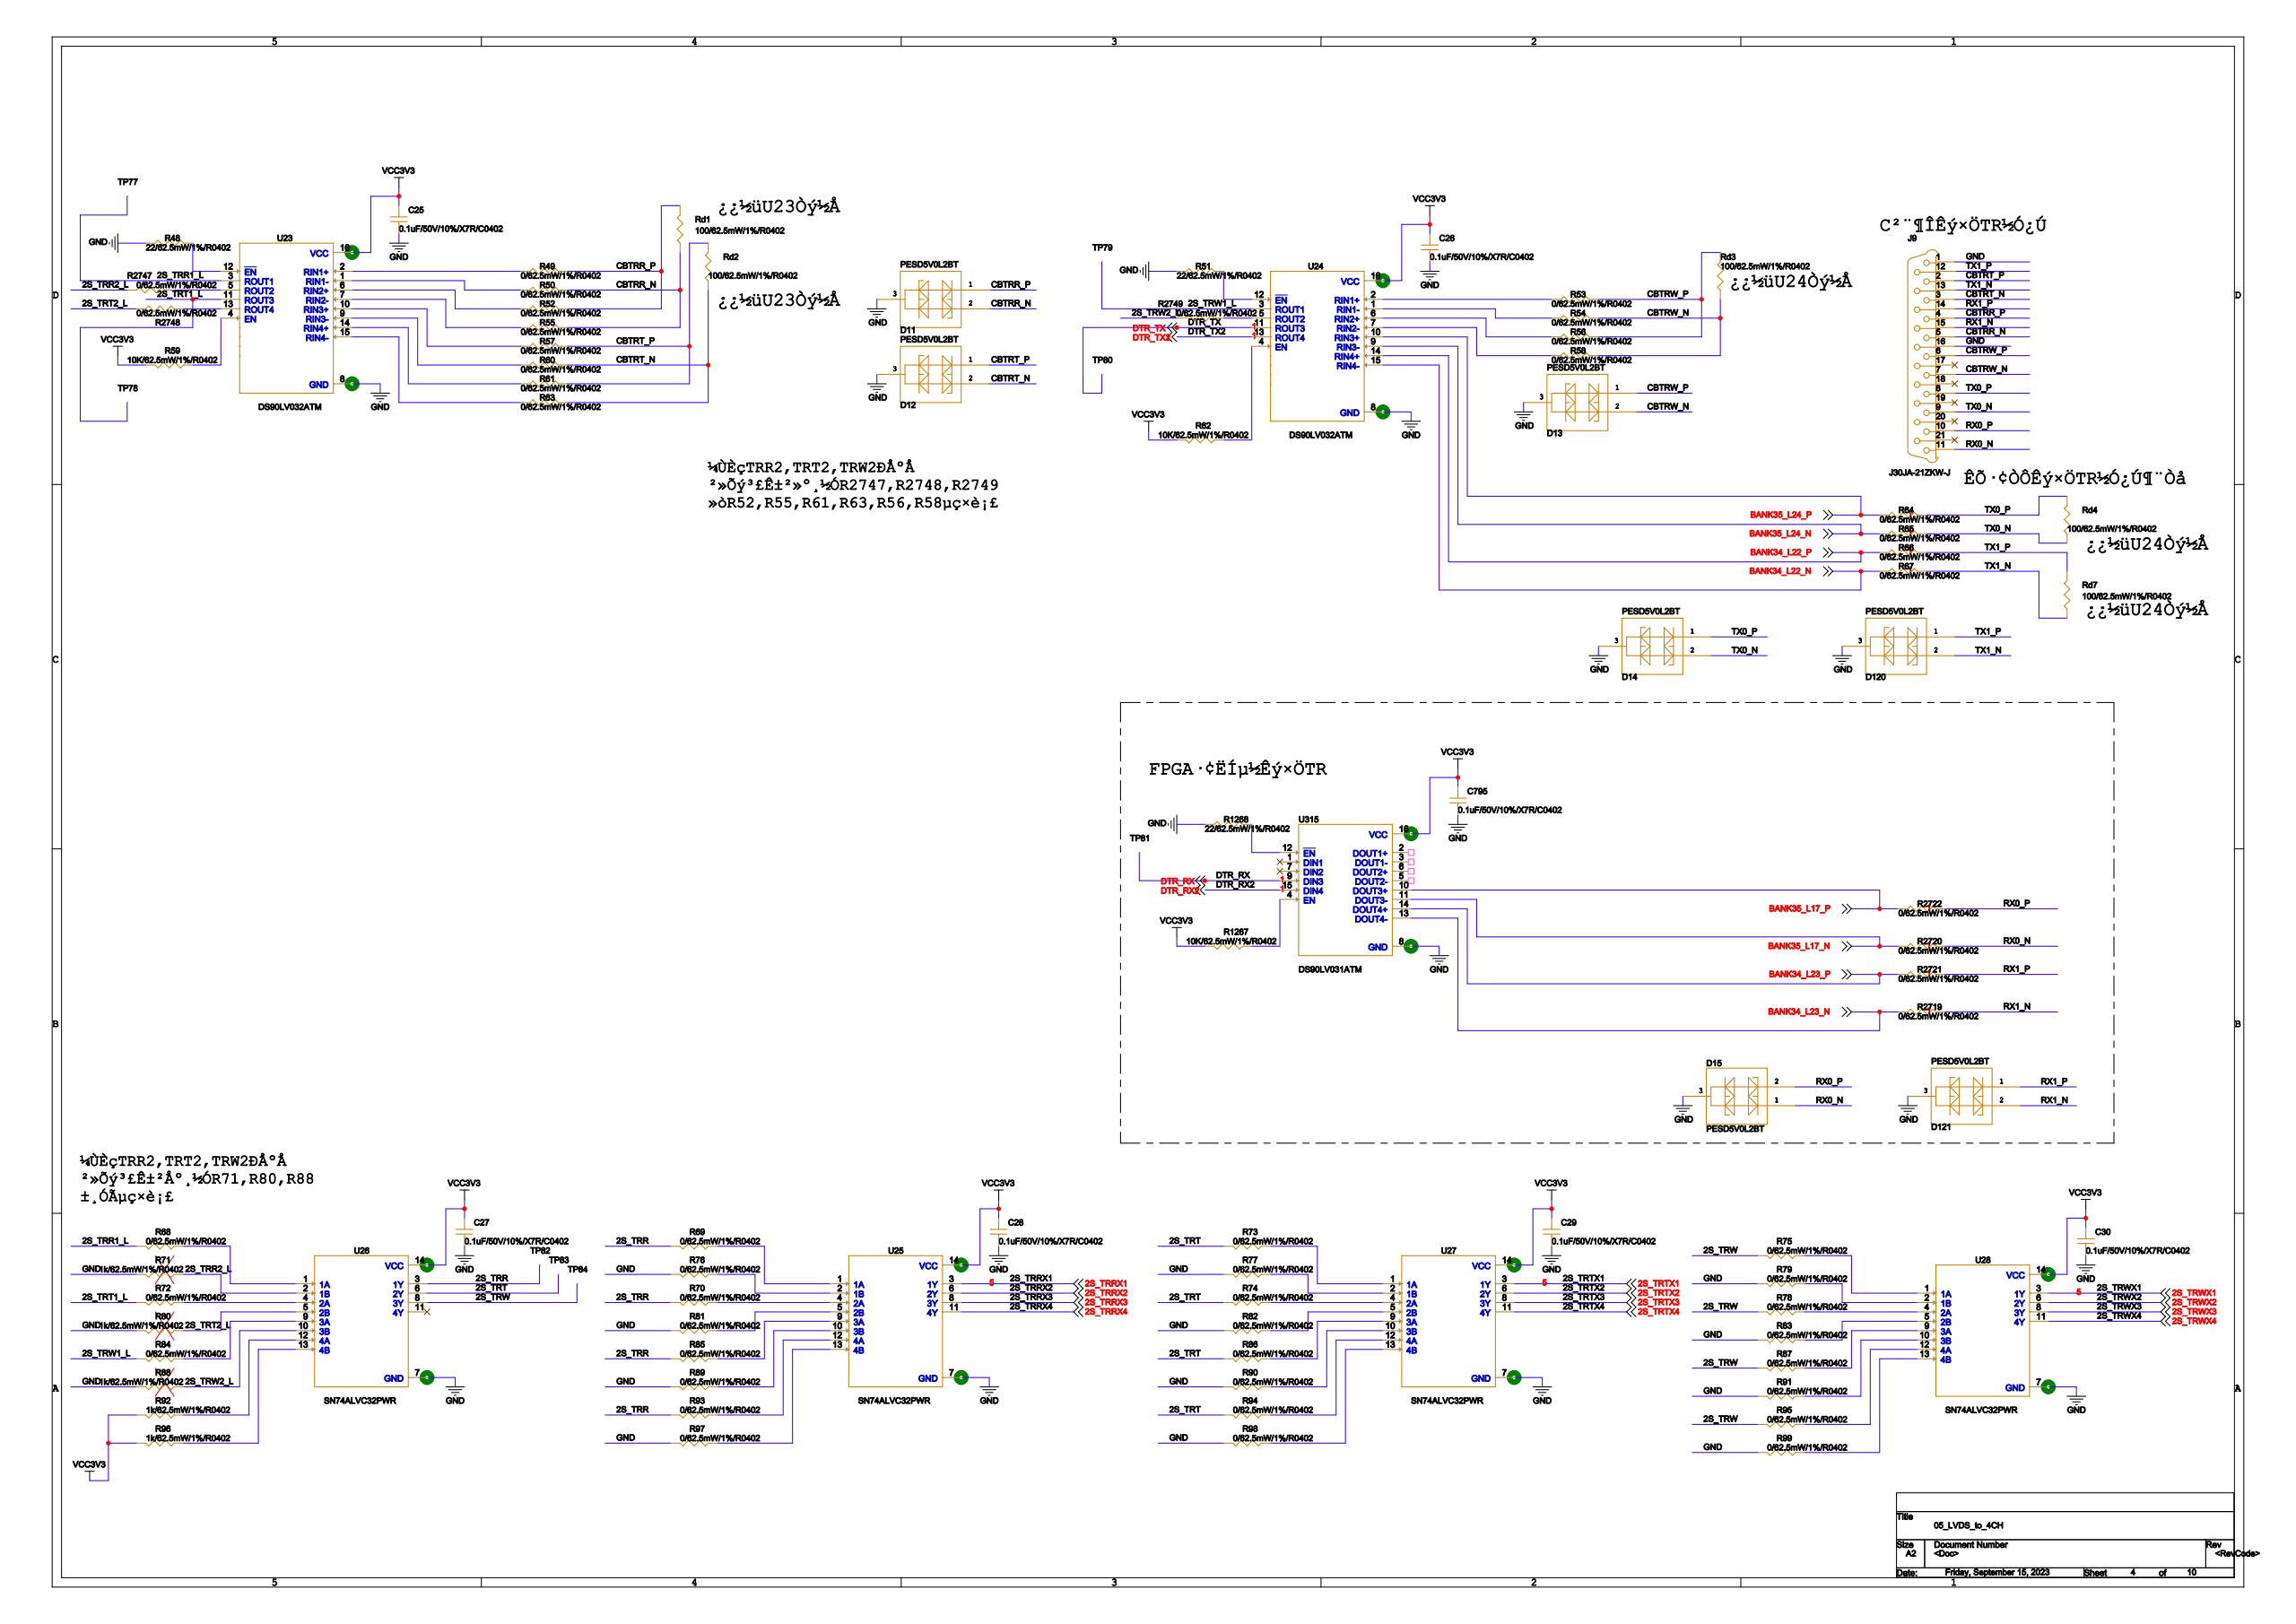Circuit board | Cadence Allegro | 634 parts | 645 nets | one sheet of the schematic
Parts on this sheet (reference | value | footprint):
C25 | 0.1uF/50V/10%/X7R/C0402 | 0402
C26 | 0.1uF/50V/10%/X7R/C0402 | 0402
C27 | 0.1uF/50V/10%/X7R/C0402 | 0402
C28 | 0.1uF/50V/10%/X7R/C0402 | 0402
C29 | 0.1uF/50V/10%/X7R/C0402 | 0402
C30 | 0.1uF/50V/10%/X7R/C0402 | 0402
C795 | 0.1uF/50V/10%/X7R/C0402 | 0402
D11 | PESD5V0L2BT | SOT23
D12 | PESD5V0L2BT | SOT23
D13 | PESD5V0L2BT | SOT23
D14 | PESD5V0L2BT | SOT23
D15 | PESD5V0L2BT | SOT23
D120 | PESD5V0L2BT | SOT23
D121 | PESD5V0L2BT | SOT23
J9 | J30JA-21ZKW-J | J30JA-21ZKW-J
R48 | 22/62.5mW/1%/R0402 | 0402
R49 | 0/62.5mW/1%/R0402 | 0402
R50 | 0/62.5mW/1%/R0402 | 0402
R51 | 22/62.5mW/1%/R0402 | 0402
R52 | 0/62.5mW/1%/R0402 | 0402
R53 | 0/62.5mW/1%/R0402 | 0402
R54 | 0/62.5mW/1%/R0402 | 0402
R55 | 0/62.5mW/1%/R0402 | 0402
R56 | 0/62.5mW/1%/R0402 | 0402
R57 | 0/62.5mW/1%/R0402 | 0402
R58 | 0/62.5mW/1%/R0402 | 0402
R59 | 10K/62.5mW/1%/R0402 | 0402
R60 | 0/62.5mW/1%/R0402 | 0402
R61 | 0/62.5mW/1%/R0402 | 0402
R62 | 10K/62.5mW/1%/R0402 | 0402
R63 | 0/62.5mW/1%/R0402 | 0402
R64 | 0/62.5mW/1%/R0402 | 0402
R65 | 0/62.5mW/1%/R0402 | 0402
R66 | 0/62.5mW/1%/R0402 | 0402
R67 | 0/62.5mW/1%/R0402 | 0402
R68 | 0/62.5mW/1%/R0402 | 0402
R69 | 0/62.5mW/1%/R0402 | 0402
R70 | 0/62.5mW/1%/R0402 | 0402
R71 | 1k/62.5mW/1%/R0402 | 0402
R72 | 0/62.5mW/1%/R0402 | 0402
R73 | 0/62.5mW/1%/R0402 | 0402
R74 | 0/62.5mW/1%/R0402 | 0402
R75 | 0/62.5mW/1%/R0402 | 0402
R76 | 0/62.5mW/1%/R0402 | 0402
R77 | 0/62.5mW/1%/R0402 | 0402
R78 | 0/62.5mW/1%/R0402 | 0402
R79 | 0/62.5mW/1%/R0402 | 0402
R80 | 1k/62.5mW/1%/R0402 | 0402
R81 | 0/62.5mW/1%/R0402 | 0402
R82 | 0/62.5mW/1%/R0402 | 0402
R83 | 0/62.5mW/1%/R0402 | 0402
R84 | 0/62.5mW/1%/R0402 | 0402
R85 | 0/62.5mW/1%/R0402 | 0402
R86 | 0/62.5mW/1%/R0402 | 0402
R87 | 0/62.5mW/1%/R0402 | 0402
R88 | 1k/62.5mW/1%/R0402 | 0402
R89 | 0/62.5mW/1%/R0402 | 0402
R90 | 0/62.5mW/1%/R0402 | 0402
R91 | 0/62.5mW/1%/R0402 | 0402
R92 | 1k/62.5mW/1%/R0402 | 0402
R93 | 0/62.5mW/1%/R0402 | 0402
R94 | 0/62.5mW/1%/R0402 | 0402
R95 | 0/62.5mW/1%/R0402 | 0402
R96 | 1k/62.5mW/1%/R0402 | 0402
R97 | 0/62.5mW/1%/R0402 | 0402
R98 | 0/62.5mW/1%/R0402 | 0402
R99 | 0/62.5mW/1%/R0402 | 0402
R1267 | 10K/62.5mW/1%/R0402 | 0402
R1268 | 22/62.5mW/1%/R0402 | 0402
R2719 | 0/62.5mW/1%/R0402 | 0402
R2720 | 0/62.5mW/1%/R0402 | 0402
R2721 | 0/62.5mW/1%/R0402 | 0402
R2722 | 0/62.5mW/1%/R0402 | 0402
R2747 | 0/62.5mW/1%/R0402 | 0402
R2748 | 0/62.5mW/1%/R0402 | 0402
R2749 | 0/62.5mW/1%/R0402 | 0402
TP77 | TEST POINT A | TEST_12MM
TP78 | TEST POINT A | TEST_12MM
TP79 | TEST POINT A | TEST_12MM
TP80 | TEST POINT A | TEST_12MM
TP81 | TEST POINT A | TEST_12MM
TP82 | TEST POINT A | TEST_12MM
TP83 | TEST POINT A | TEST_12MM
TP84 | TEST POINT A | TEST_12MM
U23 | DS90LV032ATM | SOIC127P600X175-16N
U24 | DS90LV032ATM | SOIC127P600X175-16N
U25 | SN74ALVC32PWR | SOP65P640X120-14N
U26 | SN74ALVC32PWR | SOP65P640X120-14N
U27 | SN74ALVC32PWR | SOP65P640X120-14N
U28 | SN74ALVC32PWR | SOP65P640X120-14N
U315 | DS90LV031ATM | SOIC127P600X175-16N
Nets of these parts (net: part-pin ...):
AGND: C25-2 C26-2 C27-2 C28-2 C29-2 C30-2 C795-2 D11-3 D12-3 D13-3 D14-3 D15-3 D120-3 D121-3 J9-1 J9-16 R48-2 R51-2 R71-1 R76-1 R77-1 R79-1 R80-1 R81-1 R82-1 R83-1 R88-1 R89-1 R90-1 R91-1 R97-1 R98-1 R99-1 R1268-2 U23-8 U24-8 U25-7 U26-7 U27-7 U28-7 U315-8
DTR_TX: TP80-1 U24-11
3.3V: C25-1 C26-1 C27-1 C28-1 C29-1 C30-1 C795-1 R59-1 R62-1 R92-1 R96-1 R1267-1 U23-16 U24-16 U25-14 U26-14 U27-14 U28-14 U315-16
DTR_TX2: U24-13
DTR_RX: TP81-1 U315-9
DTR_RX2: U315-15
BANK34_L23_P: R2721-2 U315-14
BANK34_L23_N: R2719-2 U315-13
BANK35_L17_P: R2722-2 U315-10
BANK35_L17_N: R2720-2 U315-11
BANK35_L24_P: R64-2 U24-10
BANK35_L24_N: R65-2 U24-9
BANK34_L22_P: R66-2 U24-14
BANK34_L22_N: R67-2 U24-15
2S_TRR2_L: R71-2 R2747-2 U26-2
2S_TRT2_L: R80-2 R2748-2 U26-5
2S_TRW2_L: R88-2 R2749-2 U26-10
N23948082: R92-2 U26-12
N23948113: R96-2 U26-13
N24593317: R1267-2 U315-4
N24593321: R1268-1 U315-12
TX1_P: D120-1 J9-12 R66-1
TX1_N: D120-2 J9-13 R67-1
CBTRR_P: D11-1 J9-4 R49-1 R52-1
CBTRR_N: D11-2 J9-5 R50-1 R55-1
CBTRT_P: D12-1 J9-2 R57-1 R61-1
CBTRT_N: D12-2 J9-3 R60-1 R63-1
CBTRW_P: D13-1 J9-6 R53-1 R56-1
CBTRW_N: D13-2 J9-7 R54-1 R58-1
TX0_P: D14-1 J9-8 R64-1
TX0_N: D14-2 J9-9 R65-1
RX0_P: D15-2 J9-10 R2722-1
RX0_N: D15-1 J9-11 R2720-1
RX1_P: D121-1 J9-14 R2721-1
RX1_N: D121-2 J9-15 R2719-1
N24594376: R2747-1 U23-5
N24594406: R2748-1 U23-13
N24594432: R2749-1 U24-5
2S_TRRX1: U25-3
2S_TRTX1: U27-3
2S_TRWX1: U28-3
N23932828: R49-2 U23-2
N23932816: R50-2 U23-1
N23932818: R52-2 U23-6
N23933318: R53-2 U24-2
N23933306: R54-2 U24-1
N23932814: R55-2 U23-7
N23933308: R56-2 U24-6
N23932880: R57-2 U23-10
N23933304: R58-2 U24-7
N23932860: R60-2 U23-9
N23932862: R61-2 U23-14
N23932858: R63-2 U23-15
2S_TRR1_L: R68-1 TP77-1 U23-3
N23947474: R68-2 U26-1
2S_TRR: R69-1 R70-1 R85-1 R93-1 TP82-1 U26-3
N23951252: R69-2 U25-1
N23951241: R70-2 U25-4
2S_TRT1_L: R72-1 TP78-1 U23-11
N23947464: R72-2 U26-4
2S_TRT: R73-1 R74-1 R86-1 R94-1 TP83-1 U26-6
N23952028: R73-2 U27-1
N23952017: R74-2 U27-4
2S_TRW: R75-1 R78-1 R87-1 R95-1 TP84-1 U26-8
N23952637: R75-2 U28-1
N23951246: R76-2 U25-2
N23952022: R77-2 U27-2
N23952626: R78-2 U28-4
N23952631: R79-2 U28-2
N23951235: R81-2 U25-5
N23952011: R82-2 U27-5
N23952620: R83-2 U28-5
2S_TRW1_L: R84-1 TP79-1 U24-3
N23947916: R84-2 U26-9
N23951299: R85-2 U25-9
N23952075: R86-2 U27-9
N23952684: R87-2 U28-9
N23951313: R89-2 U25-10
N23952089: R90-2 U27-10
N23952698: R91-2 U28-10
N23951333: R93-2 U25-12
N23952098: R94-2 U27-12
N23952707: R95-2 U28-12
N23951346: R97-2 U25-13
N23952119: R98-2 U27-13
N23952728: R99-2 U28-13
N23932768: R59-2 U23-4
N23932772: R48-1 U23-12
N23933268: R62-2 U24-4
N23933272: R51-1 U24-12
2S_TRRX2: U25-6
2S_TRRX3: U25-8
2S_TRRX4: U25-11
2S_TRTX2: U27-6
2S_TRTX3: U27-8
2S_TRTX4: U27-11
2S_TRWX2: U28-6
2S_TRWX3: U28-8
2S_TRWX4: U28-11